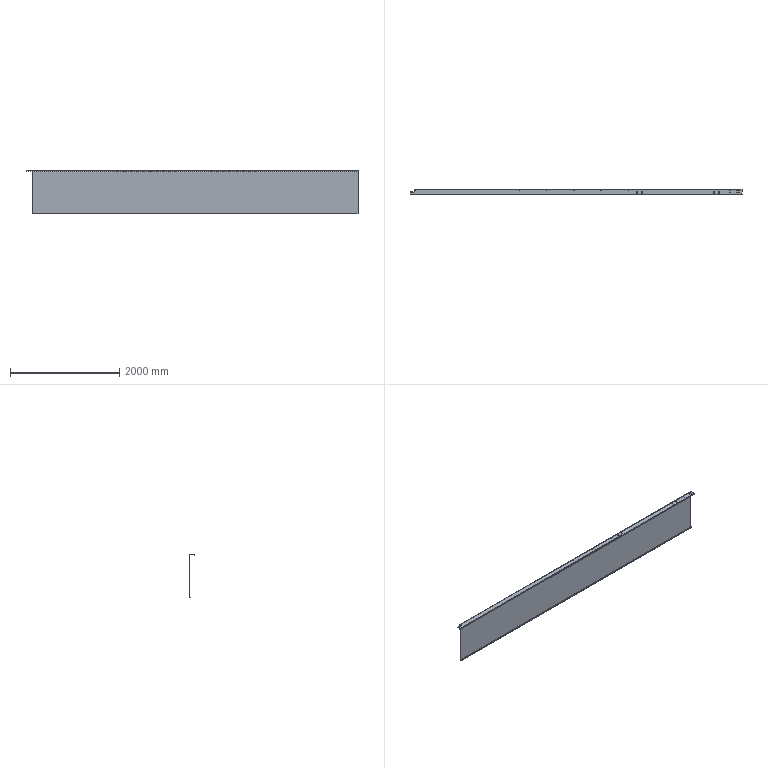Part | STEP file | Microwave Drying Flat Conveyor-CN2500x400-103-101a | 1 solid | 102 faces | box 6084 x 93 x 803 mm | volume 16530711 mm3 | cylinder 76 | plane 25 | spline 1 | commonest cylinder face diameters 6 x27 9 x16 11 x16 7 x10 12 x3 20 x2